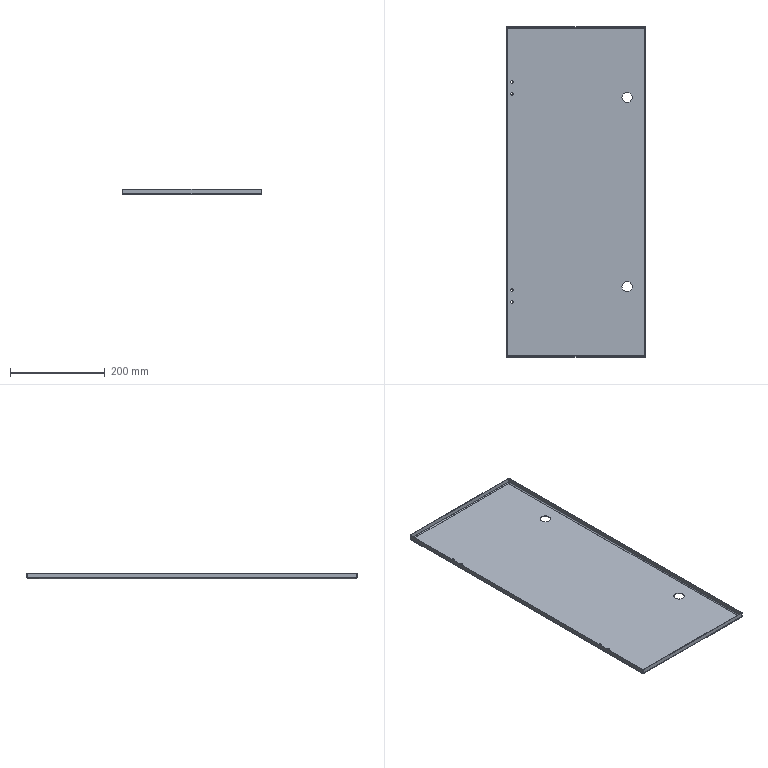Part | STEP file | Vertical arm rear door (default) | 1 solid | 78 faces | box 296 x 698 x 12 mm | volume 225434 mm3 | plane 34 | cylinder 24 | spline 20 | commonest cylinder face diameters 5.5 x8 2 x4 4 x4 6 x4 22 x4